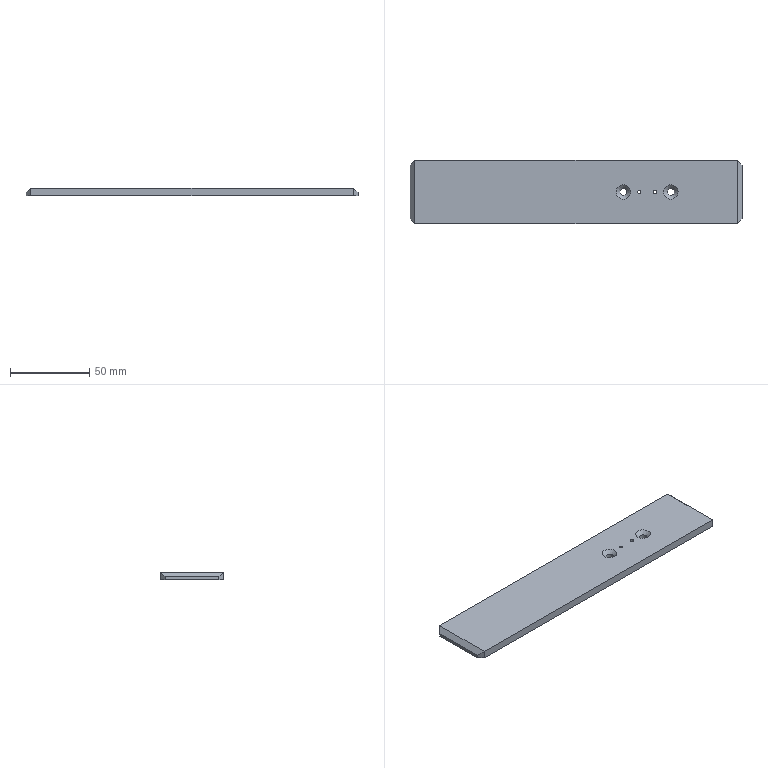Part | STEP file | Tube feed_id782_x_t | 1 solid | 18 faces | box 210 x 40 x 5 mm | volume 41286 mm3 | plane 12 | cylinder 4 | cone 2 | commonest cylinder face diameters 2 x2 4.6 x2
STEP:
#1=CARTESIAN_POINT('',(0.,0.,0.));
#2=DIRECTION('',(0.,0.,1.));
#3=DIRECTION('',(1.,0.,0.));
#4=AXIS2_PLACEMENT_3D('',#1,#2,#3);
#5=CARTESIAN_POINT('',(354.3,10.036,-6.));
#6=VERTEX_POINT('',#5);
#7=CARTESIAN_POINT('',(349.7,10.036,-6.));
#8=VERTEX_POINT('',#7);
#9=CARTESIAN_POINT('',(352.,10.036,-6.));
#10=DIRECTION('',(0.,0.,1.));
#11=DIRECTION('',(1.,0.,0.));
#12=AXIS2_PLACEMENT_3D('',#9,#10,#11);
#13=CIRCLE('',#12,2.3);
#14=CARTESIAN_POINT('',(0.,0.,-6.));
#15=DIRECTION('',(0.,0.,1.));
#16=DIRECTION('',(1.,0.,0.));
#17=AXIS2_PLACEMENT_3D('',#14,#15,#16);
#18=PLANE('',#17);
#19=CARTESIAN_POINT('',(352.,10.036));
#20=DIRECTION('',(1.,0.));
#21=AXIS2_PLACEMENT_2D('',#19,#20);
#22=CIRCLE('',#21,2.3);
#23=(GEOMETRIC_REPRESENTATION_CONTEXT(2)PARAMETRIC_REPRESENTATION_CONTEXT()REPRESENTATION_CONTEXT('',''));
#24=DEFINITIONAL_REPRESENTATION('',(#22),#23);
#25=PCURVE('',#18,#24);
#26=CARTESIAN_POINT('',(352.,10.036,-17.3));
#27=DIRECTION('',(0.,0.,-1.));
#28=DIRECTION('',(-1.,0.,0.));
#29=AXIS2_PLACEMENT_3D('',#26,#27,#28);
#30=CYLINDRICAL_SURFACE('',#29,2.3);
#31=CARTESIAN_POINT('',(3.142,-11.3));
#32=DIRECTION('',(-1.,0.));
#33=VECTOR('',#32,1.);
#34=LINE('',#31,#33);
#35=(GEOMETRIC_REPRESENTATION_CONTEXT(2)PARAMETRIC_REPRESENTATION_CONTEXT()REPRESENTATION_CONTEXT('',''));
#36=DEFINITIONAL_REPRESENTATION('',(#34),#35);
#37=PCURVE('',#30,#36);
#38=SURFACE_CURVE('',#13,(#25,#37),.PCURVE_S1.);
#39=EDGE_CURVE('',#6,#8,#38,.T.);
#40=ORIENTED_EDGE('',*,*,#39,.T.);
#41=CARTESIAN_POINT('',(352.,10.036,-6.));
#42=DIRECTION('',(0.,0.,1.));
#43=DIRECTION('',(1.,0.,0.));
#44=AXIS2_PLACEMENT_3D('',#41,#42,#43);
#45=CIRCLE('',#44,2.3);
#46=CARTESIAN_POINT('',(352.,10.036));
#47=DIRECTION('',(1.,0.));
#48=AXIS2_PLACEMENT_2D('',#46,#47);
#49=CIRCLE('',#48,2.3);
#50=(GEOMETRIC_REPRESENTATION_CONTEXT(2)PARAMETRIC_REPRESENTATION_CONTEXT()REPRESENTATION_CONTEXT('',''));
#51=DEFINITIONAL_REPRESENTATION('',(#49),#50);
#52=PCURVE('',#18,#51);
#53=CARTESIAN_POINT('',(9.425,-11.3));
#54=DIRECTION('',(-1.,0.));
#55=VECTOR('',#54,1.);
#56=LINE('',#53,#55);
#57=(GEOMETRIC_REPRESENTATION_CONTEXT(2)PARAMETRIC_REPRESENTATION_CONTEXT()REPRESENTATION_CONTEXT('',''));
#58=DEFINITIONAL_REPRESENTATION('',(#56),#57);
#59=PCURVE('',#30,#58);
#60=SURFACE_CURVE('',#45,(#52,#59),.PCURVE_S1.);
#61=EDGE_CURVE('',#8,#6,#60,.T.);
#62=ORIENTED_EDGE('',*,*,#61,.T.);
#63=EDGE_LOOP('',(#40,#62));
#64=FACE_BOUND('',#63,.T.);
#65=CARTESIAN_POINT('',(343.,10.036,-6.));
#66=VERTEX_POINT('',#65);
#67=CARTESIAN_POINT('',(342.,10.036,-6.));
#68=DIRECTION('',(0.,0.,1.));
#69=DIRECTION('',(1.,0.,0.));
#70=AXIS2_PLACEMENT_3D('',#67,#68,#69);
#71=CIRCLE('',#70,1.);
#72=CARTESIAN_POINT('',(342.,10.036));
#73=DIRECTION('',(1.,0.));
#74=AXIS2_PLACEMENT_2D('',#72,#73);
#75=CIRCLE('',#74,1.);
#76=(GEOMETRIC_REPRESENTATION_CONTEXT(2)PARAMETRIC_REPRESENTATION_CONTEXT()REPRESENTATION_CONTEXT('',''));
#77=DEFINITIONAL_REPRESENTATION('',(#75),#76);
#78=PCURVE('',#18,#77);
#79=CARTESIAN_POINT('',(342.,10.036,-21.));
#80=DIRECTION('',(0.,0.,-1.));
#81=DIRECTION('',(-1.,0.,0.));
#82=AXIS2_PLACEMENT_3D('',#79,#80,#81);
#83=CYLINDRICAL_SURFACE('',#82,1.);
#84=CARTESIAN_POINT('',(9.425,-15.));
#85=DIRECTION('',(-1.,0.));
#86=VECTOR('',#85,1.);
#87=LINE('',#84,#86);
#88=(GEOMETRIC_REPRESENTATION_CONTEXT(2)PARAMETRIC_REPRESENTATION_CONTEXT()REPRESENTATION_CONTEXT('',''));
#89=DEFINITIONAL_REPRESENTATION('',(#87),#88);
#90=PCURVE('',#83,#89);
#91=SURFACE_CURVE('',#71,(#78,#90),.PCURVE_S1.);
#92=EDGE_CURVE('',#66,#66,#91,.T.);
#93=ORIENTED_EDGE('',*,*,#92,.T.);
#94=EDGE_LOOP('',(#93));
#95=FACE_BOUND('',#94,.T.);
#96=CARTESIAN_POINT('',(333.,10.036,-6.));
#97=VERTEX_POINT('',#96);
#98=CARTESIAN_POINT('',(332.,10.036,-6.));
#99=DIRECTION('',(0.,0.,1.));
#100=DIRECTION('',(1.,0.,0.));
#101=AXIS2_PLACEMENT_3D('',#98,#99,#100);
#102=CIRCLE('',#101,1.);
#103=CARTESIAN_POINT('',(332.,10.036));
#104=DIRECTION('',(1.,0.));
#105=AXIS2_PLACEMENT_2D('',#103,#104);
#106=CIRCLE('',#105,1.);
#107=(GEOMETRIC_REPRESENTATION_CONTEXT(2)PARAMETRIC_REPRESENTATION_CONTEXT()REPRESENTATION_CONTEXT('',''));
#108=DEFINITIONAL_REPRESENTATION('',(#106),#107);
#109=PCURVE('',#18,#108);
#110=CARTESIAN_POINT('',(332.,10.036,-21.));
#111=DIRECTION('',(0.,0.,-1.));
#112=DIRECTION('',(-1.,0.,0.));
#113=AXIS2_PLACEMENT_3D('',#110,#111,#112);
#114=CYLINDRICAL_SURFACE('',#113,1.);
#115=CARTESIAN_POINT('',(9.425,-15.));
#116=DIRECTION('',(-1.,0.));
#117=VECTOR('',#116,1.);
#118=LINE('',#115,#117);
#119=(GEOMETRIC_REPRESENTATION_CONTEXT(2)PARAMETRIC_REPRESENTATION_CONTEXT()REPRESENTATION_CONTEXT('',''));
#120=DEFINITIONAL_REPRESENTATION('',(#118),#119);
#121=PCURVE('',#114,#120);
#122=SURFACE_CURVE('',#102,(#109,#121),.PCURVE_S1.);
#123=EDGE_CURVE('',#97,#97,#122,.T.);
#124=ORIENTED_EDGE('',*,*,#123,.T.);
#125=EDGE_LOOP('',(#124));
#126=FACE_BOUND('',#125,.T.);
#127=CARTESIAN_POINT('',(190.,-9.964,-6.));
#128=VERTEX_POINT('',#127);
#129=CARTESIAN_POINT('',(394.,-9.964,-6.));
#130=VERTEX_POINT('',#129);
#131=CARTESIAN_POINT('',(187.,-9.964,-6.));
#132=DIRECTION('',(1.,0.,0.));
#133=VECTOR('',#132,1.);
#134=LINE('',#131,#133);
#135=CARTESIAN_POINT('',(187.,-9.964));
#136=DIRECTION('',(1.,0.));
#137=VECTOR('',#136,1.);
#138=LINE('',#135,#137);
#139=(GEOMETRIC_REPRESENTATION_CONTEXT(2)PARAMETRIC_REPRESENTATION_CONTEXT()REPRESENTATION_CONTEXT('',''));
#140=DEFINITIONAL_REPRESENTATION('',(#138),#139);
#141=PCURVE('',#18,#140);
#142=CARTESIAN_POINT('',(187.,-9.964,-1.));
#143=DIRECTION('',(0.,1.,0.));
#144=DIRECTION('',(0.,0.,1.));
#145=AXIS2_PLACEMENT_3D('',#142,#143,#144);
#146=PLANE('',#145);
#147=CARTESIAN_POINT('',(-5.,0.));
#148=DIRECTION('',(0.,1.));
#149=VECTOR('',#148,1.);
#150=LINE('',#147,#149);
#151=(GEOMETRIC_REPRESENTATION_CONTEXT(2)PARAMETRIC_REPRESENTATION_CONTEXT()REPRESENTATION_CONTEXT('',''));
#152=DEFINITIONAL_REPRESENTATION('',(#150),#151);
#153=PCURVE('',#146,#152);
#154=SURFACE_CURVE('',#134,(#141,#153),.PCURVE_S1.);
#155=EDGE_CURVE('',#128,#130,#154,.T.);
#156=ORIENTED_EDGE('',*,*,#155,.F.);
#157=CARTESIAN_POINT('',(187.,-6.964,-6.));
#158=VERTEX_POINT('',#157);
#159=CARTESIAN_POINT('',(190.,-9.964,-6.));
#160=DIRECTION('',(-0.7071,0.7071,0.));
#161=VECTOR('',#160,1.);
#162=LINE('',#159,#161);
#163=CARTESIAN_POINT('',(190.,-9.964));
#164=DIRECTION('',(-0.7071,0.7071));
#165=VECTOR('',#164,1.);
#166=LINE('',#163,#165);
#167=(GEOMETRIC_REPRESENTATION_CONTEXT(2)PARAMETRIC_REPRESENTATION_CONTEXT()REPRESENTATION_CONTEXT('',''));
#168=DEFINITIONAL_REPRESENTATION('',(#166),#167);
#169=PCURVE('',#18,#168);
#170=CARTESIAN_POINT('',(190.,-9.964,-1.));
#171=DIRECTION('',(0.7071,0.7071,0.));
#172=DIRECTION('',(0.,0.,-1.));
#173=AXIS2_PLACEMENT_3D('',#170,#171,#172);
#174=PLANE('',#173);
#175=CARTESIAN_POINT('',(5.,0.));
#176=DIRECTION('',(0.,1.));
#177=VECTOR('',#176,1.);
#178=LINE('',#175,#177);
#179=(GEOMETRIC_REPRESENTATION_CONTEXT(2)PARAMETRIC_REPRESENTATION_CONTEXT()REPRESENTATION_CONTEXT('',''));
#180=DEFINITIONAL_REPRESENTATION('',(#178),#179);
#181=PCURVE('',#174,#180);
#182=SURFACE_CURVE('',#162,(#169,#181),.PCURVE_S1.);
#183=EDGE_CURVE('',#128,#158,#182,.T.);
#184=ORIENTED_EDGE('',*,*,#183,.T.);
#185=CARTESIAN_POINT('',(187.,27.036,-6.));
#186=VERTEX_POINT('',#185);
#187=CARTESIAN_POINT('',(187.,30.036,-6.));
#188=DIRECTION('',(0.,-1.,0.));
#189=VECTOR('',#188,1.);
#190=LINE('',#187,#189);
#191=CARTESIAN_POINT('',(187.,30.036));
#192=DIRECTION('',(0.,-1.));
#193=VECTOR('',#192,1.);
#194=LINE('',#191,#193);
#195=(GEOMETRIC_REPRESENTATION_CONTEXT(2)PARAMETRIC_REPRESENTATION_CONTEXT()REPRESENTATION_CONTEXT('',''));
#196=DEFINITIONAL_REPRESENTATION('',(#194),#195);
#197=PCURVE('',#18,#196);
#198=CARTESIAN_POINT('',(187.,30.036,-1.));
#199=DIRECTION('',(1.,0.,0.));
#200=DIRECTION('',(0.,0.,-1.));
#201=AXIS2_PLACEMENT_3D('',#198,#199,#200);
#202=PLANE('',#201);
#203=CARTESIAN_POINT('',(5.,0.));
#204=DIRECTION('',(0.,-1.));
#205=VECTOR('',#204,1.);
#206=LINE('',#203,#205);
#207=(GEOMETRIC_REPRESENTATION_CONTEXT(2)PARAMETRIC_REPRESENTATION_CONTEXT()REPRESENTATION_CONTEXT('',''));
#208=DEFINITIONAL_REPRESENTATION('',(#206),#207);
#209=PCURVE('',#202,#208);
#210=SURFACE_CURVE('',#190,(#197,#209),.PCURVE_S1.);
#211=EDGE_CURVE('',#186,#158,#210,.T.);
#212=ORIENTED_EDGE('',*,*,#211,.F.);
#213=CARTESIAN_POINT('',(190.,30.036,-6.));
#214=VERTEX_POINT('',#213);
#215=CARTESIAN_POINT('',(187.,27.036,-6.));
#216=DIRECTION('',(0.7071,0.7071,0.));
#217=VECTOR('',#216,1.);
#218=LINE('',#215,#217);
#219=CARTESIAN_POINT('',(187.,27.036));
#220=DIRECTION('',(0.7071,0.7071));
#221=VECTOR('',#220,1.);
#222=LINE('',#219,#221);
#223=(GEOMETRIC_REPRESENTATION_CONTEXT(2)PARAMETRIC_REPRESENTATION_CONTEXT()REPRESENTATION_CONTEXT('',''));
#224=DEFINITIONAL_REPRESENTATION('',(#222),#223);
#225=PCURVE('',#18,#224);
#226=CARTESIAN_POINT('',(187.,27.036,-1.));
#227=DIRECTION('',(0.7071,-0.7071,0.));
#228=DIRECTION('',(0.,0.,-1.));
#229=AXIS2_PLACEMENT_3D('',#226,#227,#228);
#230=PLANE('',#229);
#231=CARTESIAN_POINT('',(5.,0.));
#232=DIRECTION('',(0.,1.));
#233=VECTOR('',#232,1.);
#234=LINE('',#231,#233);
#235=(GEOMETRIC_REPRESENTATION_CONTEXT(2)PARAMETRIC_REPRESENTATION_CONTEXT()REPRESENTATION_CONTEXT('',''));
#236=DEFINITIONAL_REPRESENTATION('',(#234),#235);
#237=PCURVE('',#230,#236);
#238=SURFACE_CURVE('',#218,(#225,#237),.PCURVE_S1.);
#239=EDGE_CURVE('',#186,#214,#238,.T.);
#240=ORIENTED_EDGE('',*,*,#239,.T.);
#241=CARTESIAN_POINT('',(394.,30.036,-6.));
#242=VERTEX_POINT('',#241);
#243=CARTESIAN_POINT('',(397.,30.036,-6.));
#244=DIRECTION('',(-1.,0.,0.));
#245=VECTOR('',#244,1.);
#246=LINE('',#243,#245);
#247=CARTESIAN_POINT('',(397.,30.036));
#248=DIRECTION('',(-1.,0.));
#249=VECTOR('',#248,1.);
#250=LINE('',#247,#249);
#251=(GEOMETRIC_REPRESENTATION_CONTEXT(2)PARAMETRIC_REPRESENTATION_CONTEXT()REPRESENTATION_CONTEXT('',''));
#252=DEFINITIONAL_REPRESENTATION('',(#250),#251);
#253=PCURVE('',#18,#252);
#254=CARTESIAN_POINT('',(397.,30.036,-1.));
#255=DIRECTION('',(0.,-1.,0.));
#256=DIRECTION('',(0.,0.,-1.));
#257=AXIS2_PLACEMENT_3D('',#254,#255,#256);
#258=PLANE('',#257);
#259=CARTESIAN_POINT('',(5.,0.));
#260=DIRECTION('',(0.,-1.));
#261=VECTOR('',#260,1.);
#262=LINE('',#259,#261);
#263=(GEOMETRIC_REPRESENTATION_CONTEXT(2)PARAMETRIC_REPRESENTATION_CONTEXT()REPRESENTATION_CONTEXT('',''));
#264=DEFINITIONAL_REPRESENTATION('',(#262),#263);
#265=PCURVE('',#258,#264);
#266=SURFACE_CURVE('',#246,(#253,#265),.PCURVE_S1.);
#267=EDGE_CURVE('',#242,#214,#266,.T.);
#268=ORIENTED_EDGE('',*,*,#267,.F.);
#269=CARTESIAN_POINT('',(397.,27.036,-6.));
#270=VERTEX_POINT('',#269);
#271=CARTESIAN_POINT('',(394.,30.036,-6.));
#272=DIRECTION('',(0.7071,-0.7071,0.));
#273=VECTOR('',#272,1.);
#274=LINE('',#271,#273);
#275=CARTESIAN_POINT('',(394.,30.036));
#276=DIRECTION('',(0.7071,-0.7071));
#277=VECTOR('',#276,1.);
#278=LINE('',#275,#277);
#279=(GEOMETRIC_REPRESENTATION_CONTEXT(2)PARAMETRIC_REPRESENTATION_CONTEXT()REPRESENTATION_CONTEXT('',''));
#280=DEFINITIONAL_REPRESENTATION('',(#278),#279);
#281=PCURVE('',#18,#280);
#282=CARTESIAN_POINT('',(394.,30.036,-1.));
#283=DIRECTION('',(-0.7071,-0.7071,0.));
#284=DIRECTION('',(0.,0.,-1.));
#285=AXIS2_PLACEMENT_3D('',#282,#283,#284);
#286=PLANE('',#285);
#287=CARTESIAN_POINT('',(5.,0.));
#288=DIRECTION('',(0.,1.));
#289=VECTOR('',#288,1.);
#290=LINE('',#287,#289);
#291=(GEOMETRIC_REPRESENTATION_CONTEXT(2)PARAMETRIC_REPRESENTATION_CONTEXT()REPRESENTATION_CONTEXT('',''));
#292=DEFINITIONAL_REPRESENTATION('',(#290),#291);
#293=PCURVE('',#286,#292);
#294=SURFACE_CURVE('',#274,(#281,#293),.PCURVE_S1.);
#295=EDGE_CURVE('',#242,#270,#294,.T.);
#296=ORIENTED_EDGE('',*,*,#295,.T.);
#297=CARTESIAN_POINT('',(397.,-6.964,-6.));
#298=VERTEX_POINT('',#297);
#299=CARTESIAN_POINT('',(397.,-9.964,-6.));
#300=DIRECTION('',(0.,1.,0.));
#301=VECTOR('',#300,1.);
#302=LINE('',#299,#301);
#303=CARTESIAN_POINT('',(397.,-9.964));
#304=DIRECTION('',(0.,1.));
#305=VECTOR('',#304,1.);
#306=LINE('',#303,#305);
#307=(GEOMETRIC_REPRESENTATION_CONTEXT(2)PARAMETRIC_REPRESENTATION_CONTEXT()REPRESENTATION_CONTEXT('',''));
#308=DEFINITIONAL_REPRESENTATION('',(#306),#307);
#309=PCURVE('',#18,#308);
#310=CARTESIAN_POINT('',(397.,-9.964,-1.));
#311=DIRECTION('',(-1.,0.,0.));
#312=DIRECTION('',(0.,0.,1.));
#313=AXIS2_PLACEMENT_3D('',#310,#311,#312);
#314=PLANE('',#313);
#315=CARTESIAN_POINT('',(-5.,0.));
#316=DIRECTION('',(0.,1.));
#317=VECTOR('',#316,1.);
#318=LINE('',#315,#317);
#319=(GEOMETRIC_REPRESENTATION_CONTEXT(2)PARAMETRIC_REPRESENTATION_CONTEXT()REPRESENTATION_CONTEXT('',''));
#320=DEFINITIONAL_REPRESENTATION('',(#318),#319);
#321=PCURVE('',#314,#320);
#322=SURFACE_CURVE('',#302,(#309,#321),.PCURVE_S1.);
#323=EDGE_CURVE('',#298,#270,#322,.T.);
#324=ORIENTED_EDGE('',*,*,#323,.F.);
#325=CARTESIAN_POINT('',(397.,-6.964,-6.));
#326=DIRECTION('',(-0.7071,-0.7071,0.));
#327=VECTOR('',#326,1.);
#328=LINE('',#325,#327);
#329=CARTESIAN_POINT('',(397.,-6.964));
#330=DIRECTION('',(-0.7071,-0.7071));
#331=VECTOR('',#330,1.);
#332=LINE('',#329,#331);
#333=(GEOMETRIC_REPRESENTATION_CONTEXT(2)PARAMETRIC_REPRESENTATION_CONTEXT()REPRESENTATION_CONTEXT('',''));
#334=DEFINITIONAL_REPRESENTATION('',(#332),#333);
#335=PCURVE('',#18,#334);
#336=CARTESIAN_POINT('',(397.,-6.964,-1.));
#337=DIRECTION('',(-0.7071,0.7071,0.));
#338=DIRECTION('',(0.,0.,-1.));
#339=AXIS2_PLACEMENT_3D('',#336,#337,#338);
#340=PLANE('',#339);
#341=CARTESIAN_POINT('',(5.,0.));
#342=DIRECTION('',(0.,1.));
#343=VECTOR('',#342,1.);
#344=LINE('',#341,#343);
#345=(GEOMETRIC_REPRESENTATION_CONTEXT(2)PARAMETRIC_REPRESENTATION_CONTEXT()REPRESENTATION_CONTEXT('',''));
#346=DEFINITIONAL_REPRESENTATION('',(#344),#345);
#347=PCURVE('',#340,#346);
#348=SURFACE_CURVE('',#328,(#335,#347),.PCURVE_S1.);
#349=EDGE_CURVE('',#298,#130,#348,.T.);
#350=ORIENTED_EDGE('',*,*,#349,.T.);
#351=EDGE_LOOP('',(#156,#184,#212,#240,#268,#296,#324,#350));
#352=FACE_BOUND('',#351,.T.);
#353=CARTESIAN_POINT('',(324.3,10.036,-6.));
#354=VERTEX_POINT('',#353);
#355=CARTESIAN_POINT('',(319.7,10.036,-6.));
#356=VERTEX_POINT('',#355);
#357=CARTESIAN_POINT('',(322.,10.036,-6.));
#358=DIRECTION('',(0.,0.,1.));
#359=DIRECTION('',(1.,0.,0.));
#360=AXIS2_PLACEMENT_3D('',#357,#358,#359);
#361=CIRCLE('',#360,2.3);
#362=CARTESIAN_POINT('',(322.,10.036));
#363=DIRECTION('',(1.,0.));
#364=AXIS2_PLACEMENT_2D('',#362,#363);
#365=CIRCLE('',#364,2.3);
#366=(GEOMETRIC_REPRESENTATION_CONTEXT(2)PARAMETRIC_REPRESENTATION_CONTEXT()REPRESENTATION_CONTEXT('',''));
#367=DEFINITIONAL_REPRESENTATION('',(#365),#366);
#368=PCURVE('',#18,#367);
#369=CARTESIAN_POINT('',(322.,10.036,-17.3));
#370=DIRECTION('',(0.,0.,-1.));
#371=DIRECTION('',(-1.,0.,0.));
#372=AXIS2_PLACEMENT_3D('',#369,#370,#371);
#373=CYLINDRICAL_SURFACE('',#372,2.3);
#374=CARTESIAN_POINT('',(3.142,-11.3));
#375=DIRECTION('',(-1.,0.));
#376=VECTOR('',#375,1.);
#377=LINE('',#374,#376);
#378=(GEOMETRIC_REPRESENTATION_CONTEXT(2)PARAMETRIC_REPRESENTATION_CONTEXT()REPRESENTATION_CONTEXT('',''));
#379=DEFINITIONAL_REPRESENTATION('',(#377),#378);
#380=PCURVE('',#373,#379);
#381=SURFACE_CURVE('',#361,(#368,#380),.PCURVE_S1.);
#382=EDGE_CURVE('',#354,#356,#381,.T.);
#383=ORIENTED_EDGE('',*,*,#382,.T.);
#384=CARTESIAN_POINT('',(322.,10.036,-6.));
#385=DIRECTION('',(0.,0.,1.));
#386=DIRECTION('',(1.,0.,0.));
#387=AXIS2_PLACEMENT_3D('',#384,#385,#386);
#388=CIRCLE('',#387,2.3);
#389=CARTESIAN_POINT('',(322.,10.036));
#390=DIRECTION('',(1.,0.));
#391=AXIS2_PLACEMENT_2D('',#389,#390);
#392=CIRCLE('',#391,2.3);
#393=(GEOMETRIC_REPRESENTATION_CONTEXT(2)PARAMETRIC_REPRESENTATION_CONTEXT()REPRESENTATION_CONTEXT('',''));
#394=DEFINITIONAL_REPRESENTATION('',(#392),#393);
#395=PCURVE('',#18,#394);
#396=CARTESIAN_POINT('',(9.425,-11.3));
#397=DIRECTION('',(-1.,0.));
#398=VECTOR('',#397,1.);
#399=LINE('',#396,#398);
#400=(GEOMETRIC_REPRESENTATION_CONTEXT(2)PARAMETRIC_REPRESENTATION_CONTEXT()REPRESENTATION_CONTEXT('',''));
#401=DEFINITIONAL_REPRESENTATION('',(#399),#400);
#402=PCURVE('',#373,#401);
#403=SURFACE_CURVE('',#388,(#395,#402),.PCURVE_S1.);
#404=EDGE_CURVE('',#356,#354,#403,.T.);
#405=ORIENTED_EDGE('',*,*,#404,.T.);
#406=EDGE_LOOP('',(#383,#405));
#407=FACE_BOUND('',#406,.T.);
#408=ADVANCED_FACE('',(#64,#95,#126,#352,#407),#18,.F.);
#409=ORIENTED_EDGE('',*,*,#211,.T.);
#410=CARTESIAN_POINT('',(187.,-6.964,-4.));
#411=VERTEX_POINT('',#410);
#412=CARTESIAN_POINT('',(187.,-6.964,-1.));
#413=DIRECTION('',(0.,0.,1.));
#414=VECTOR('',#413,1.);
#415=LINE('',#412,#414);
#416=CARTESIAN_POINT('',(0.,-37.));
#417=DIRECTION('',(-1.,0.));
#418=VECTOR('',#417,1.);
#419=LINE('',#416,#418);
#420=(GEOMETRIC_REPRESENTATION_CONTEXT(2)PARAMETRIC_REPRESENTATION_CONTEXT()REPRESENTATION_CONTEXT('',''));
#421=DEFINITIONAL_REPRESENTATION('',(#419),#420);
#422=PCURVE('',#202,#421);
#423=CARTESIAN_POINT('',(0.,4.243));
#424=DIRECTION('',(-1.,0.));
#425=VECTOR('',#424,1.);
#426=LINE('',#423,#425);
#427=(GEOMETRIC_REPRESENTATION_CONTEXT(2)PARAMETRIC_REPRESENTATION_CONTEXT()REPRESENTATION_CONTEXT('',''));
#428=DEFINITIONAL_REPRESENTATION('',(#426),#427);
#429=PCURVE('',#174,#428);
#430=SURFACE_CURVE('',#415,(#422,#429),.PCURVE_S1.);
#431=EDGE_CURVE('',#158,#411,#430,.T.);
#432=ORIENTED_EDGE('',*,*,#431,.T.);
#433=CARTESIAN_POINT('',(187.,27.036,-4.));
#434=VERTEX_POINT('',#433);
#435=CARTESIAN_POINT('',(187.,30.036,-4.));
#436=DIRECTION('',(0.,1.,0.));
#437=VECTOR('',#436,1.);
#438=LINE('',#435,#437);
#439=CARTESIAN_POINT('',(3.,0.));
#440=DIRECTION('',(0.,1.));
#441=VECTOR('',#440,1.);
#442=LINE('',#439,#441);
#443=(GEOMETRIC_REPRESENTATION_CONTEXT(2)PARAMETRIC_REPRESENTATION_CONTEXT()REPRESENTATION_CONTEXT('',''));
#444=DEFINITIONAL_REPRESENTATION('',(#442),#443);
#445=PCURVE('',#202,#444);
#446=CARTESIAN_POINT('',(190.,0.,-1.));
#447=DIRECTION('',(-0.7071,0.,0.7071));
#448=DIRECTION('',(0.,1.,0.));
#449=AXIS2_PLACEMENT_3D('',#446,#447,#448);
#450=PLANE('',#449);
#451=CARTESIAN_POINT('',(30.036,4.243));
#452=DIRECTION('',(1.,0.));
#453=VECTOR('',#452,1.);
#454=LINE('',#451,#453);
#455=(GEOMETRIC_REPRESENTATION_CONTEXT(2)PARAMETRIC_REPRESENTATION_CONTEXT()REPRESENTATION_CONTEXT('',''));
#456=DEFINITIONAL_REPRESENTATION('',(#454),#455);
#457=PCURVE('',#450,#456);
#458=SURFACE_CURVE('',#438,(#445,#457),.PCURVE_S1.);
#459=EDGE_CURVE('',#411,#434,#458,.T.);
#460=ORIENTED_EDGE('',*,*,#459,.T.);
#461=CARTESIAN_POINT('',(187.,27.036,-1.));
#462=DIRECTION('',(0.,0.,-1.));
#463=VECTOR('',#462,1.);
#464=LINE('',#461,#463);
#465=CARTESIAN_POINT('',(0.,-3.));
#466=DIRECTION('',(1.,0.));
#467=VECTOR('',#466,1.);
#468=LINE('',#465,#467);
#469=(GEOMETRIC_REPRESENTATION_CONTEXT(2)PARAMETRIC_REPRESENTATION_CONTEXT()REPRESENTATION_CONTEXT('',''));
#470=DEFINITIONAL_REPRESENTATION('',(#468),#469);
#471=PCURVE('',#202,#470);
#472=CARTESIAN_POINT('',(0.,0.));
#473=DIRECTION('',(1.,0.));
#474=VECTOR('',#473,1.);
#475=LINE('',#472,#474);
#476=(GEOMETRIC_REPRESENTATION_CONTEXT(2)PARAMETRIC_REPRESENTATION_CONTEXT()REPRESENTATION_CONTEXT('',''));
#477=DEFINITIONAL_REPRESENTATION('',(#475),#476);
#478=PCURVE('',#230,#477);
#479=SURFACE_CURVE('',#464,(#471,#478),.PCURVE_S1.);
#480=EDGE_CURVE('',#434,#186,#479,.T.);
#481=ORIENTED_EDGE('',*,*,#480,.T.);
#482=EDGE_LOOP('',(#409,#432,#460,#481));
#483=FACE_BOUND('',#482,.T.);
#484=ADVANCED_FACE('',(#483),#202,.F.);
#485=CARTESIAN_POINT('',(190.,-9.964,-1.));
#486=VERTEX_POINT('',#485);
#487=CARTESIAN_POINT('',(394.,-9.964,-1.));
#488=VERTEX_POINT('',#487);
#489=CARTESIAN_POINT('',(187.,-9.964,-1.));
#490=DIRECTION('',(1.,0.,0.));
#491=VECTOR('',#490,1.);
#492=LINE('',#489,#491);
#493=CARTESIAN_POINT('',(0.,0.));
#494=DIRECTION('',(0.,1.));
#495=VECTOR('',#494,1.);
#496=LINE('',#493,#495);
#497=(GEOMETRIC_REPRESENTATION_CONTEXT(2)PARAMETRIC_REPRESENTATION_CONTEXT()REPRESENTATION_CONTEXT('',''));
#498=DEFINITIONAL_REPRESENTATION('',(#496),#497);
#499=PCURVE('',#146,#498);
#500=CARTESIAN_POINT('',(0.,0.,-1.));
#501=DIRECTION('',(0.,0.,1.));
#502=DIRECTION('',(1.,0.,0.));
#503=AXIS2_PLACEMENT_3D('',#500,#501,#502);
#504=PLANE('',#503);
#505=CARTESIAN_POINT('',(187.,-9.964));
#506=DIRECTION('',(1.,0.));
#507=VECTOR('',#506,1.);
#508=LINE('',#505,#507);
#509=(GEOMETRIC_REPRESENTATION_CONTEXT(2)PARAMETRIC_REPRESENTATION_CONTEXT()REPRESENTATION_CONTEXT('',''));
#510=DEFINITIONAL_REPRESENTATION('',(#508),#509);
#511=PCURVE('',#504,#510);
#512=SURFACE_CURVE('',#492,(#499,#511),.PCURVE_S1.);
#513=EDGE_CURVE('',#486,#488,#512,.T.);
#514=ORIENTED_EDGE('',*,*,#513,.F.);
#515=CARTESIAN_POINT('',(190.,-9.964,-1.));
#516=DIRECTION('',(0.,0.,-1.));
#517=VECTOR('',#516,1.);
#518=LINE('',#515,#517);
#519=CARTESIAN_POINT('',(0.,3.));
#520=DIRECTION('',(-1.,0.));
#521=VECTOR('',#520,1.);
#522=LINE('',#519,#521);
#523=(GEOMETRIC_REPRESENTATION_CONTEXT(2)PARAMETRIC_REPRESENTATION_CONTEXT()REPRESENTATION_CONTEXT('',''));
#524=DEFINITIONAL_REPRESENTATION('',(#522),#523);
#525=PCURVE('',#146,#524);
#526=CARTESIAN_POINT('',(0.,0.));
#527=DIRECTION('',(1.,0.));
#528=VECTOR('',#527,1.);
#529=LINE('',#526,#528);
#530=(GEOMETRIC_REPRESENTATION_CONTEXT(2)PARAMETRIC_REPRESENTATION_CONTEXT()REPRESENTATION_CONTEXT('',''));
#531=DEFINITIONAL_REPRESENTATION('',(#529),#530);
#532=PCURVE('',#174,#531);
#533=SURFACE_CURVE('',#518,(#525,#532),.PCURVE_S1.);
#534=EDGE_CURVE('',#486,#128,#533,.T.);
#535=ORIENTED_EDGE('',*,*,#534,.T.);
#536=ORIENTED_EDGE('',*,*,#155,.T.);
#537=CARTESIAN_POINT('',(394.,-9.964,-1.));
#538=DIRECTION('',(0.,0.,1.));
#539=VECTOR('',#538,1.);
#540=LINE('',#537,#539);
#541=CARTESIAN_POINT('',(0.,207.));
#542=DIRECTION('',(1.,0.));
#543=VECTOR('',#542,1.);
#544=LINE('',#541,#543);
#545=(GEOMETRIC_REPRESENTATION_CONTEXT(2)PARAMETRIC_REPRESENTATION_CONTEXT()REPRESENTATION_CONTEXT('',''));
#546=DEFINITIONAL_REPRESENTATION('',(#544),#545);
#547=PCURVE('',#146,#546);
#548=CARTESIAN_POINT('',(0.,4.243));
#549=DIRECTION('',(-1.,0.));
#550=VECTOR('',#549,1.);
#551=LINE('',#548,#550);
#552=(GEOMETRIC_REPRESENTATION_CONTEXT(2)PARAMETRIC_REPRESENTATION_CONTEXT()REPRESENTATION_CONTEXT('',''));
#553=DEFINITIONAL_REPRESENTATION('',(#551),#552);
#554=PCURVE('',#340,#553);
#555=SURFACE_CURVE('',#540,(#547,#554),.PCURVE_S1.);
#556=EDGE_CURVE('',#130,#488,#555,.T.);
#557=ORIENTED_EDGE('',*,*,#556,.T.);
#558=EDGE_LOOP('',(#514,#535,#536,#557));
#559=FACE_BOUND('',#558,.T.);
#560=ADVANCED_FACE('',(#559),#146,.F.);
#561=CARTESIAN_POINT('',(397.,27.036,-4.));
#562=VERTEX_POINT('',#561);
#563=CARTESIAN_POINT('',(397.,-6.964,-4.));
#564=VERTEX_POINT('',#563);
#565=CARTESIAN_POINT('',(397.,-9.964,-4.));
#566=DIRECTION('',(0.,-1.,0.));
#567=VECTOR('',#566,1.);
#568=LINE('',#565,#567);
#569=CARTESIAN_POINT('',(-3.,0.));
#570=DIRECTION('',(0.,-1.));
#571=VECTOR('',#570,1.);
#572=LINE('',#569,#571);
#573=(GEOMETRIC_REPRESENTATION_CONTEXT(2)PARAMETRIC_REPRESENTATION_CONTEXT()REPRESENTATION_CONTEXT('',''));
#574=DEFINITIONAL_REPRESENTATION('',(#572),#573);
#575=PCURVE('',#314,#574);
#576=CARTESIAN_POINT('',(394.,0.,-1.));
#577=DIRECTION('',(0.7071,0.,0.7071));
#578=DIRECTION('',(0.,-1.,0.));
#579=AXIS2_PLACEMENT_3D('',#576,#577,#578);
#580=PLANE('',#579);
#581=CARTESIAN_POINT('',(9.964,4.243));
#582=DIRECTION('',(1.,0.));
#583=VECTOR('',#582,1.);
#584=LINE('',#581,#583);
#585=(GEOMETRIC_REPRESENTATION_CONTEXT(2)PARAMETRIC_REPRESENTATION_CONTEXT()REPRESENTATION_CONTEXT('',''));
#586=DEFINITIONAL_REPRESENTATION('',(#584),#585);
#587=PCURVE('',#580,#586);
#588=SURFACE_CURVE('',#568,(#575,#587),.PCURVE_S1.);
#589=EDGE_CURVE('',#562,#564,#588,.T.);
#590=ORIENTED_EDGE('',*,*,#589,.T.);
#591=CARTESIAN_POINT('',(397.,-6.964,-1.));
#592=DIRECTION('',(0.,0.,-1.));
#593=VECTOR('',#592,1.);
#594=LINE('',#591,#593);
#595=CARTESIAN_POINT('',(0.,3.));
#596=DIRECTION('',(-1.,0.));
#597=VECTOR('',#596,1.);
#598=LINE('',#595,#597);
#599=(GEOMETRIC_REPRESENTATION_CONTEXT(2)PARAMETRIC_REPRESENTATION_CONTEXT()REPRESENTATION_CONTEXT('',''));
#600=DEFINITIONAL_REPRESENTATION('',(#598),#599);
#601=PCURVE('',#314,#600);
#602=CARTESIAN_POINT('',(0.,0.));
#603=DIRECTION('',(1.,0.));
#604=VECTOR('',#603,1.);
#605=LINE('',#602,#604);
#606=(GEOMETRIC_REPRESENTATION_CONTEXT(2)PARAMETRIC_REPRESENTATION_CONTEXT()REPRESENTATION_CONTEXT('',''));
#607=DEFINITIONAL_REPRESENTATION('',(#605),#606);
#608=PCURVE('',#340,#607);
#609=SURFACE_CURVE('',#594,(#601,#608),.PCURVE_S1.);
#610=EDGE_CURVE('',#564,#298,#609,.T.);
#611=ORIENTED_EDGE('',*,*,#610,.T.);
#612=ORIENTED_EDGE('',*,*,#323,.T.);
#613=CARTESIAN_POINT('',(397.,27.036,-1.));
#614=DIRECTION('',(0.,0.,1.));
#615=VECTOR('',#614,1.);
#616=LINE('',#613,#615);
#617=CARTESIAN_POINT('',(0.,37.));
#618=DIRECTION('',(1.,0.));
#619=VECTOR('',#618,1.);
#620=LINE('',#617,#619);
#621=(GEOMETRIC_REPRESENTATION_CONTEXT(2)PARAMETRIC_REPRESENTATION_CONTEXT()REPRESENTATION_CONTEXT('',''));
#622=DEFINITIONAL_REPRESENTATION('',(#620),#621);
#623=PCURVE('',#314,#622);
#624=CARTESIAN_POINT('',(0.,4.243));
#625=DIRECTION('',(-1.,0.));
#626=VECTOR('',#625,1.);
#627=LINE('',#624,#626);
#628=(GEOMETRIC_REPRESENTATION_CONTEXT(2)PARAMETRIC_REPRESENTATION_CONTEXT()REPRESENTATION_CONTEXT('',''));
#629=DEFINITIONAL_REPRESENTATION('',(#627),#628);
#630=PCURVE('',#286,#629);
#631=SURFACE_CURVE('',#616,(#623,#630),.PCURVE_S1.);
#632=EDGE_CURVE('',#270,#562,#631,.T.);
#633=ORIENTED_EDGE('',*,*,#632,.T.);
#634=EDGE_LOOP('',(#590,#611,#612,#633));
#635=FACE_BOUND('',#634,.T.);
#636=ADVANCED_FACE('',(#635),#314,.F.);
#637=ORIENTED_EDGE('',*,*,#267,.T.);
#638=CARTESIAN_POINT('',(190.,30.036,-1.));
#639=VERTEX_POINT('',#638);
#640=CARTESIAN_POINT('',(190.,30.036,-1.));
#641=DIRECTION('',(0.,0.,1.));
#642=VECTOR('',#641,1.);
#643=LINE('',#640,#642);
#644=CARTESIAN_POINT('',(0.,-207.));
#645=DIRECTION('',(-1.,0.));
#646=VECTOR('',#645,1.);
#647=LINE('',#644,#646);
#648=(GEOMETRIC_REPRESENTATION_CONTEXT(2)PARAMETRIC_REPRESENTATION_CONTEXT()REPRESENTATION_CONTEXT('',''));
#649=DEFINITIONAL_REPRESENTATION('',(#647),#648);
#650=PCURVE('',#258,#649);
#651=CARTESIAN_POINT('',(0.,4.243));
#652=DIRECTION('',(-1.,0.));
#653=VECTOR('',#652,1.);
#654=LINE('',#651,#653);
#655=(GEOMETRIC_REPRESENTATION_CONTEXT(2)PARAMETRIC_REPRESENTATION_CONTEXT()REPRESENTATION_CONTEXT('',''));
#656=DEFINITIONAL_REPRESENTATION('',(#654),#655);
#657=PCURVE('',#230,#656);
#658=SURFACE_CURVE('',#643,(#650,#657),.PCURVE_S1.);
#659=EDGE_CURVE('',#214,#639,#658,.T.);
#660=ORIENTED_EDGE('',*,*,#659,.T.);
#661=CARTESIAN_POINT('',(394.,30.036,-1.));
#662=VERTEX_POINT('',#661);
#663=CARTESIAN_POINT('',(397.,30.036,-1.));
#664=DIRECTION('',(-1.,0.,0.));
#665=VECTOR('',#664,1.);
#666=LINE('',#663,#665);
#667=CARTESIAN_POINT('',(0.,0.));
#668=DIRECTION('',(0.,-1.));
#669=VECTOR('',#668,1.);
#670=LINE('',#667,#669);
#671=(GEOMETRIC_REPRESENTATION_CONTEXT(2)PARAMETRIC_REPRESENTATION_CONTEXT()REPRESENTATION_CONTEXT('',''));
#672=DEFINITIONAL_REPRESENTATION('',(#670),#671);
#673=PCURVE('',#258,#672);
#674=CARTESIAN_POINT('',(397.,30.036));
#675=DIRECTION('',(-1.,0.));
#676=VECTOR('',#675,1.);
#677=LINE('',#674,#676);
#678=(GEOMETRIC_REPRESENTATION_CONTEXT(2)PARAMETRIC_REPRESENTATION_CONTEXT()REPRESENTATION_CONTEXT('',''));
#679=DEFINITIONAL_REPRESENTATION('',(#677),#678);
#680=PCURVE('',#504,#679);
#681=SURFACE_CURVE('',#666,(#673,#680),.PCURVE_S1.);
#682=EDGE_CURVE('',#662,#639,#681,.T.);
#683=ORIENTED_EDGE('',*,*,#682,.F.);
#684=CARTESIAN_POINT('',(394.,30.036,-1.));
#685=DIRECTION('',(0.,0.,-1.));
#686=VECTOR('',#685,1.);
#687=LINE('',#684,#686);
#688=CARTESIAN_POINT('',(0.,-3.));
#689=DIRECTION('',(1.,0.));
#690=VECTOR('',#689,1.);
#691=LINE('',#688,#690);
#692=(GEOMETRIC_REPRESENTATION_CONTEXT(2)PARAMETRIC_REPRESENTATION_CONTEXT()REPRESENTATION_CONTEXT('',''));
#693=DEFINITIONAL_REPRESENTATION('',(#691),#692);
#694=PCURVE('',#258,#693);
#695=CARTESIAN_POINT('',(0.,0.));
#696=DIRECTION('',(1.,0.));
#697=VECTOR('',#696,1.);
#698=LINE('',#695,#697);
#699=(GEOMETRIC_REPRESENTATION_CONTEXT(2)PARAMETRIC_REPRESENTATION_CONTEXT()REPRESENTATION_CONTEXT('',''));
#700=DEFINITIONAL_REPRESENTATION('',(#698),#699);
#701=PCURVE('',#286,#700);
#702=SURFACE_CURVE('',#687,(#694,#701),.PCURVE_S1.);
#703=EDGE_CURVE('',#662,#242,#702,.T.);
#704=ORIENTED_EDGE('',*,*,#703,.T.);
#705=EDGE_LOOP('',(#637,#660,#683,#704));
#706=FACE_BOUND('',#705,.T.);
#707=ADVANCED_FACE('',(#706),#258,.F.);
#708=CARTESIAN_POINT('',(347.4,10.036,-1.));
#709=VERTEX_POINT('',#708);
#710=CARTESIAN_POINT('',(352.,10.036,-1.));
#711=DIRECTION('',(0.,0.,-1.));
#712=DIRECTION('',(-1.,0.,0.));
#713=AXIS2_PLACEMENT_3D('',#710,#711,#712);
#714=CIRCLE('',#713,4.6);
#715=CARTESIAN_POINT('',(347.4,10.036));
#716=CARTESIAN_POINT('',(347.4,18.003));
#717=CARTESIAN_POINT('',(354.3,14.019));
#718=CARTESIAN_POINT('',(361.2,10.036));
#719=CARTESIAN_POINT('',(354.3,6.052));
#720=CARTESIAN_POINT('',(347.4,2.068));
#721=CARTESIAN_POINT('',(347.4,10.036));
#722=(BOUNDED_CURVE()B_SPLINE_CURVE(2,(#715,#716,#717,#718,#719,#720,#721),.UNSPECIFIED.,.T.,.F.)B_SPLINE_CURVE_WITH_KNOTS((1,2,2,2,2,1),(-2.094,0.,2.094,4.189,6.283,8.378),.UNSPECIFIED.)CURVE()GEOMETRIC_REPRESENTATION_ITEM()RATIONAL_B_SPLINE_CURVE((1.,0.5,1.,0.5,1.,0.5,1.))REPRESENTATION_ITEM(''));
#723=(GEOMETRIC_REPRESENTATION_CONTEXT(2)PARAMETRIC_REPRESENTATION_CONTEXT()REPRESENTATION_CONTEXT('',''));
#724=DEFINITIONAL_REPRESENTATION('',(#722),#723);
#725=PCURVE('',#504,#724);
#726=CARTESIAN_POINT('',(352.,10.036,-3.3));
#727=DIRECTION('',(0.,0.,1.));
#728=DIRECTION('',(1.,0.,0.));
#729=AXIS2_PLACEMENT_3D('',#726,#727,#728);
#730=CONICAL_SURFACE('',#729,2.3,0.7854);
#731=CARTESIAN_POINT('',(9.425,2.3));
#732=DIRECTION('',(-1.,0.));
#733=VECTOR('',#732,1.);
#734=LINE('',#731,#733);
#735=(GEOMETRIC_REPRESENTATION_CONTEXT(2)PARAMETRIC_REPRESENTATION_CONTEXT()REPRESENTATION_CONTEXT('',''));
#736=DEFINITIONAL_REPRESENTATION('',(#734),#735);
#737=PCURVE('',#730,#736);
#738=SURFACE_CURVE('',#714,(#725,#737),.PCURVE_S1.);
#739=EDGE_CURVE('',#709,#709,#738,.T.);
#740=ORIENTED_EDGE('',*,*,#739,.T.);
#741=EDGE_LOOP('',(#740));
#742=FACE_BOUND('',#741,.T.);
#743=CARTESIAN_POINT('',(317.4,10.036,-1.));
#744=VERTEX_POINT('',#743);
#745=CARTESIAN_POINT('',(322.,10.036,-1.));
#746=DIRECTION('',(0.,0.,-1.));
#747=DIRECTION('',(-1.,0.,0.));
#748=AXIS2_PLACEMENT_3D('',#745,#746,#747);
#749=CIRCLE('',#748,4.6);
#750=CARTESIAN_POINT('',(317.4,10.036));
#751=CARTESIAN_POINT('',(317.4,18.003));
#752=CARTESIAN_POINT('',(324.3,14.019));
#753=CARTESIAN_POINT('',(331.2,10.036));
#754=CARTESIAN_POINT('',(324.3,6.052));
#755=CARTESIAN_POINT('',(317.4,2.068));
#756=CARTESIAN_POINT('',(317.4,10.036));
#757=(BOUNDED_CURVE()B_SPLINE_CURVE(2,(#750,#751,#752,#753,#754,#755,#756),.UNSPECIFIED.,.T.,.F.)B_SPLINE_CURVE_WITH_KNOTS((1,2,2,2,2,1),(-2.094,0.,2.094,4.189,6.283,8.378),.UNSPECIFIED.)CURVE()GEOMETRIC_REPRESENTATION_ITEM()RATIONAL_B_SPLINE_CURVE((1.,0.5,1.,0.5,1.,0.5,1.))REPRESENTATION_ITEM(''));
#758=(GEOMETRIC_REPRESENTATION_CONTEXT(2)PARAMETRIC_REPRESENTATION_CONTEXT()REPRESENTATION_CONTEXT('',''));
#759=DEFINITIONAL_REPRESENTATION('',(#757),#758);
#760=PCURVE('',#504,#759);
#761=CARTESIAN_POINT('',(322.,10.036,-3.3));
#762=DIRECTION('',(0.,0.,1.));
#763=DIRECTION('',(1.,0.,0.));
#764=AXIS2_PLACEMENT_3D('',#761,#762,#763);
#765=CONICAL_SURFACE('',#764,2.3,0.7854);
#766=CARTESIAN_POINT('',(9.425,2.3));
#767=DIRECTION('',(-1.,0.));
#768=VECTOR('',#767,1.);
#769=LINE('',#766,#768);
#770=(GEOMETRIC_REPRESENTATION_CONTEXT(2)PARAMETRIC_REPRESENTATION_CONTEXT()REPRESENTATION_CONTEXT('',''));
#771=DEFINITIONAL_REPRESENTATION('',(#769),#770);
#772=PCURVE('',#765,#771);
#773=SURFACE_CURVE('',#749,(#760,#772),.PCURVE_S1.);
#774=EDGE_CURVE('',#744,#744,#773,.T.);
#775=ORIENTED_EDGE('',*,*,#774,.T.);
#776=EDGE_LOOP('',(#775));
#777=FACE_BOUND('',#776,.T.);
#778=CARTESIAN_POINT('',(343.,10.036,-1.));
#779=VERTEX_POINT('',#778);
#780=CARTESIAN_POINT('',(342.,10.036,-1.));
#781=DIRECTION('',(0.,0.,1.));
#782=DIRECTION('',(1.,0.,0.));
#783=AXIS2_PLACEMENT_3D('',#780,#781,#782);
#784=CIRCLE('',#783,1.);
#785=CARTESIAN_POINT('',(342.,10.036));
#786=DIRECTION('',(1.,0.));
#787=AXIS2_PLACEMENT_2D('',#785,#786);
#788=CIRCLE('',#787,1.);
#789=(GEOMETRIC_REPRESENTATION_CONTEXT(2)PARAMETRIC_REPRESENTATION_CONTEXT()REPRESENTATION_CONTEXT('',''));
#790=DEFINITIONAL_REPRESENTATION('',(#788),#789);
#791=PCURVE('',#504,#790);
#792=CARTESIAN_POINT('',(9.425,-20.));
#793=DIRECTION('',(-1.,0.));
#794=VECTOR('',#793,1.);
#795=LINE('',#792,#794);
#796=(GEOMETRIC_REPRESENTATION_CONTEXT(2)PARAMETRIC_REPRESENTATION_CONTEXT()REPRESENTATION_CONTEXT('',''));
#797=DEFINITIONAL_REPRESENTATION('',(#795),#796);
#798=PCURVE('',#83,#797);
#799=SURFACE_CURVE('',#784,(#791,#798),.PCURVE_S1.);
#800=EDGE_CURVE('',#779,#779,#799,.T.);
#801=ORIENTED_EDGE('',*,*,#800,.F.);
#802=EDGE_LOOP('',(#801));
#803=FACE_BOUND('',#802,.T.);
#804=CARTESIAN_POINT('',(333.,10.036,-1.));
#805=VERTEX_POINT('',#804);
#806=CARTESIAN_POINT('',(332.,10.036,-1.));
#807=DIRECTION('',(0.,0.,1.));
#808=DIRECTION('',(1.,0.,0.));
#809=AXIS2_PLACEMENT_3D('',#806,#807,#808);
#810=CIRCLE('',#809,1.);
#811=CARTESIAN_POINT('',(332.,10.036));
#812=DIRECTION('',(1.,0.));
#813=AXIS2_PLACEMENT_2D('',#811,#812);
#814=CIRCLE('',#813,1.);
#815=(GEOMETRIC_REPRESENTATION_CONTEXT(2)PARAMETRIC_REPRESENTATION_CONTEXT()REPRESENTATION_CONTEXT('',''));
#816=DEFINITIONAL_REPRESENTATION('',(#814),#815);
#817=PCURVE('',#504,#816);
#818=CARTESIAN_POINT('',(9.425,-20.));
#819=DIRECTION('',(-1.,0.));
#820=VECTOR('',#819,1.);
#821=LINE('',#818,#820);
#822=(GEOMETRIC_REPRESENTATION_CONTEXT(2)PARAMETRIC_REPRESENTATION_CONTEXT()REPRESENTATION_CONTEXT('',''));
#823=DEFINITIONAL_REPRESENTATION('',(#821),#822);
#824=PCURVE('',#114,#823);
#825=SURFACE_CURVE('',#810,(#817,#824),.PCURVE_S1.);
#826=EDGE_CURVE('',#805,#805,#825,.T.);
#827=ORIENTED_EDGE('',*,*,#826,.F.);
#828=EDGE_LOOP('',(#827));
#829=FACE_BOUND('',#828,.T.);
#830=ORIENTED_EDGE('',*,*,#682,.T.);
#831=CARTESIAN_POINT('',(190.,-9.964,-1.));
#832=DIRECTION('',(0.,-1.,0.));
#833=VECTOR('',#832,1.);
#834=LINE('',#831,#833);
#835=CARTESIAN_POINT('',(190.,-9.964));
#836=DIRECTION('',(0.,-1.));
#837=VECTOR('',#836,1.);
#838=LINE('',#835,#837);
#839=(GEOMETRIC_REPRESENTATION_CONTEXT(2)PARAMETRIC_REPRESENTATION_CONTEXT()REPRESENTATION_CONTEXT('',''));
#840=DEFINITIONAL_REPRESENTATION('',(#838),#839);
#841=PCURVE('',#504,#840);
#842=CARTESIAN_POINT('',(-9.964,0.));
#843=DIRECTION('',(-1.,0.));
#844=VECTOR('',#843,1.);
#845=LINE('',#842,#844);
#846=(GEOMETRIC_REPRESENTATION_CONTEXT(2)PARAMETRIC_REPRESENTATION_CONTEXT()REPRESENTATION_CONTEXT('',''));
#847=DEFINITIONAL_REPRESENTATION('',(#845),#846);
#848=PCURVE('',#450,#847);
#849=SURFACE_CURVE('',#834,(#841,#848),.PCURVE_S1.);
#850=EDGE_CURVE('',#639,#486,#849,.T.);
#851=ORIENTED_EDGE('',*,*,#850,.T.);
#852=ORIENTED_EDGE('',*,*,#513,.T.);
#853=CARTESIAN_POINT('',(394.,30.036,-1.));
#854=DIRECTION('',(0.,1.,0.));
#855=VECTOR('',#854,1.);
#856=LINE('',#853,#855);
#857=CARTESIAN_POINT('',(394.,30.036));
#858=DIRECTION('',(0.,1.));
#859=VECTOR('',#858,1.);
#860=LINE('',#857,#859);
#861=(GEOMETRIC_REPRESENTATION_CONTEXT(2)PARAMETRIC_REPRESENTATION_CONTEXT()REPRESENTATION_CONTEXT('',''));
#862=DEFINITIONAL_REPRESENTATION('',(#860),#861);
#863=PCURVE('',#504,#862);
#864=CARTESIAN_POINT('',(-30.036,0.));
#865=DIRECTION('',(-1.,0.));
#866=VECTOR('',#865,1.);
#867=LINE('',#864,#866);
#868=(GEOMETRIC_REPRESENTATION_CONTEXT(2)PARAMETRIC_REPRESENTATION_CONTEXT()REPRESENTATION_CONTEXT('',''));
#869=DEFINITIONAL_REPRESENTATION('',(#867),#868);
#870=PCURVE('',#580,#869);
#871=SURFACE_CURVE('',#856,(#863,#870),.PCURVE_S1.);
#872=EDGE_CURVE('',#488,#662,#871,.T.);
#873=ORIENTED_EDGE('',*,*,#872,.T.);
#874=EDGE_LOOP('',(#830,#851,#852,#873));
#875=FACE_BOUND('',#874,.T.);
#876=ADVANCED_FACE('',(#742,#777,#803,#829,#875),#504,.T.);
#877=ORIENTED_EDGE('',*,*,#239,.F.);
#878=ORIENTED_EDGE('',*,*,#480,.F.);
#879=CARTESIAN_POINT('',(188.,28.036,-3.));
#880=DIRECTION('',(-0.5774,-0.5774,-0.5774));
#881=VECTOR('',#880,1.);
#882=LINE('',#879,#881);
#883=CARTESIAN_POINT('',(2.,1.414));
#884=DIRECTION('',(0.5774,-0.8165));
#885=VECTOR('',#884,1.);
#886=LINE('',#883,#885);
#887=(GEOMETRIC_REPRESENTATION_CONTEXT(2)PARAMETRIC_REPRESENTATION_CONTEXT()REPRESENTATION_CONTEXT('',''));
#888=DEFINITIONAL_REPRESENTATION('',(#886),#887);
#889=PCURVE('',#230,#888);
#890=CARTESIAN_POINT('',(28.036,2.828));
#891=DIRECTION('',(-0.5774,0.8165));
#892=VECTOR('',#891,1.);
#893=LINE('',#890,#892);
#894=(GEOMETRIC_REPRESENTATION_CONTEXT(2)PARAMETRIC_REPRESENTATION_CONTEXT()REPRESENTATION_CONTEXT('',''));
#895=DEFINITIONAL_REPRESENTATION('',(#893),#894);
#896=PCURVE('',#450,#895);
#897=SURFACE_CURVE('',#882,(#889,#896),.PCURVE_S1.);
#898=EDGE_CURVE('',#639,#434,#897,.T.);
#899=ORIENTED_EDGE('',*,*,#898,.F.);
#900=ORIENTED_EDGE('',*,*,#659,.F.);
#901=EDGE_LOOP('',(#877,#878,#899,#900));
#902=FACE_BOUND('',#901,.T.);
#903=ADVANCED_FACE('',(#902),#230,.F.);
#904=ORIENTED_EDGE('',*,*,#898,.T.);
#905=ORIENTED_EDGE('',*,*,#459,.F.);
#906=CARTESIAN_POINT('',(186.679,-6.643,-4.321));
#907=DIRECTION('',(-0.5774,0.5774,-0.5774));
#908=VECTOR('',#907,1.);
#909=LINE('',#906,#908);
#910=CARTESIAN_POINT('',(-6.643,4.697));
#911=DIRECTION('',(0.5774,0.8165));
#912=VECTOR('',#911,1.);
#913=LINE('',#910,#912);
#914=(GEOMETRIC_REPRESENTATION_CONTEXT(2)PARAMETRIC_REPRESENTATION_CONTEXT()REPRESENTATION_CONTEXT('',''));
#915=DEFINITIONAL_REPRESENTATION('',(#913),#914);
#916=PCURVE('',#450,#915);
#917=CARTESIAN_POINT('',(3.321,4.697));
#918=DIRECTION('',(0.5774,0.8165));
#919=VECTOR('',#918,1.);
#920=LINE('',#917,#919);
#921=(GEOMETRIC_REPRESENTATION_CONTEXT(2)PARAMETRIC_REPRESENTATION_CONTEXT()REPRESENTATION_CONTEXT('',''));
#922=DEFINITIONAL_REPRESENTATION('',(#920),#921);
#923=PCURVE('',#174,#922);
#924=SURFACE_CURVE('',#909,(#916,#923),.PCURVE_S1.);
#925=EDGE_CURVE('',#486,#411,#924,.T.);
#926=ORIENTED_EDGE('',*,*,#925,.F.);
#927=ORIENTED_EDGE('',*,*,#850,.F.);
#928=EDGE_LOOP('',(#904,#905,#926,#927));
#929=FACE_BOUND('',#928,.T.);
#930=ADVANCED_FACE('',(#929),#450,.T.);
#931=ORIENTED_EDGE('',*,*,#925,.T.);
#932=ORIENTED_EDGE('',*,*,#431,.F.);
#933=ORIENTED_EDGE('',*,*,#183,.F.);
#934=ORIENTED_EDGE('',*,*,#534,.F.);
#935=EDGE_LOOP('',(#931,#932,#933,#934));
#936=FACE_BOUND('',#935,.T.);
#937=ADVANCED_FACE('',(#936),#174,.F.);
#938=ORIENTED_EDGE('',*,*,#295,.F.);
#939=ORIENTED_EDGE('',*,*,#703,.F.);
#940=CARTESIAN_POINT('',(404.012,20.024,-11.012));
#941=DIRECTION('',(-0.5774,0.5774,0.5774));
#942=VECTOR('',#941,1.);
#943=LINE('',#940,#942);
#944=CARTESIAN_POINT('',(10.012,14.159));
#945=DIRECTION('',(-0.5774,-0.8165));
#946=VECTOR('',#945,1.);
#947=LINE('',#944,#946);
#948=(GEOMETRIC_REPRESENTATION_CONTEXT(2)PARAMETRIC_REPRESENTATION_CONTEXT()REPRESENTATION_CONTEXT('',''));
#949=DEFINITIONAL_REPRESENTATION('',(#947),#948);
#950=PCURVE('',#286,#949);
#951=CARTESIAN_POINT('',(-20.024,14.159));
#952=DIRECTION('',(-0.5774,-0.8165));
#953=VECTOR('',#952,1.);
#954=LINE('',#951,#953);
#955=(GEOMETRIC_REPRESENTATION_CONTEXT(2)PARAMETRIC_REPRESENTATION_CONTEXT()REPRESENTATION_CONTEXT('',''));
#956=DEFINITIONAL_REPRESENTATION('',(#954),#955);
#957=PCURVE('',#580,#956);
#958=SURFACE_CURVE('',#943,(#950,#957),.PCURVE_S1.);
#959=EDGE_CURVE('',#562,#662,#958,.T.);
#960=ORIENTED_EDGE('',*,*,#959,.F.);
#961=ORIENTED_EDGE('',*,*,#632,.F.);
#962=EDGE_LOOP('',(#938,#939,#960,#961));
#963=FACE_BOUND('',#962,.T.);
#964=ADVANCED_FACE('',(#963),#286,.F.);
#965=ORIENTED_EDGE('',*,*,#959,.T.);
#966=ORIENTED_EDGE('',*,*,#872,.F.);
#967=CARTESIAN_POINT('',(397.321,-6.643,-4.321));
#968=DIRECTION('',(-0.5774,-0.5774,0.5774));
#969=VECTOR('',#968,1.);
#970=LINE('',#967,#969);
#971=CARTESIAN_POINT('',(6.643,4.697));
#972=DIRECTION('',(0.5774,-0.8165));
#973=VECTOR('',#972,1.);
#974=LINE('',#971,#973);
#975=(GEOMETRIC_REPRESENTATION_CONTEXT(2)PARAMETRIC_REPRESENTATION_CONTEXT()REPRESENTATION_CONTEXT('',''));
#976=DEFINITIONAL_REPRESENTATION('',(#974),#975);
#977=PCURVE('',#580,#976);
#978=CARTESIAN_POINT('',(3.321,-0.4546));
#979=DIRECTION('',(-0.5774,0.8165));
#980=VECTOR('',#979,1.);
#981=LINE('',#978,#980);
#982=(GEOMETRIC_REPRESENTATION_CONTEXT(2)PARAMETRIC_REPRESENTATION_CONTEXT()REPRESENTATION_CONTEXT('',''));
#983=DEFINITIONAL_REPRESENTATION('',(#981),#982);
#984=PCURVE('',#340,#983);
#985=SURFACE_CURVE('',#970,(#977,#984),.PCURVE_S1.);
#986=EDGE_CURVE('',#564,#488,#985,.T.);
#987=ORIENTED_EDGE('',*,*,#986,.F.);
#988=ORIENTED_EDGE('',*,*,#589,.F.);
#989=EDGE_LOOP('',(#965,#966,#987,#988));
#990=FACE_BOUND('',#989,.T.);
#991=ADVANCED_FACE('',(#990),#580,.T.);
#992=ORIENTED_EDGE('',*,*,#986,.T.);
#993=ORIENTED_EDGE('',*,*,#556,.F.);
#994=ORIENTED_EDGE('',*,*,#349,.F.);
#995=ORIENTED_EDGE('',*,*,#610,.F.);
#996=EDGE_LOOP('',(#992,#993,#994,#995));
#997=FACE_BOUND('',#996,.T.);
#998=ADVANCED_FACE('',(#997),#340,.F.);
#999=ORIENTED_EDGE('',*,*,#123,.T.);
#1000=CARTESIAN_POINT('',(333.,10.036,-1.));
#1001=CARTESIAN_POINT('',(333.,10.036,-6.));
#1002=B_SPLINE_CURVE_WITH_KNOTS('',1,(#1000,#1001),.UNSPECIFIED.,.F.,.F.,(2,2),(-20.,-15.),.PIECEWISE_BEZIER_KNOTS.);
#1003=CARTESIAN_POINT('',(3.142,0.));
#1004=DIRECTION('',(0.,1.));
#1005=VECTOR('',#1004,1.);
#1006=LINE('',#1003,#1005);
#1007=(GEOMETRIC_REPRESENTATION_CONTEXT(2)PARAMETRIC_REPRESENTATION_CONTEXT()REPRESENTATION_CONTEXT('',''));
#1008=DEFINITIONAL_REPRESENTATION('',(#1006),#1007);
#1009=PCURVE('',#114,#1008);
#1010=CARTESIAN_POINT('',(9.425,0.));
#1011=DIRECTION('',(0.,1.));
#1012=VECTOR('',#1011,1.);
#1013=LINE('',#1010,#1012);
#1014=(GEOMETRIC_REPRESENTATION_CONTEXT(2)PARAMETRIC_REPRESENTATION_CONTEXT()REPRESENTATION_CONTEXT('',''));
#1015=DEFINITIONAL_REPRESENTATION('',(#1013),#1014);
#1016=PCURVE('',#114,#1015);
#1017=SEAM_CURVE('',#1002,(#1009,#1016),.PCURVE_S1.);
#1018=EDGE_CURVE('',#805,#97,#1017,.T.);
#1019=ORIENTED_EDGE('',*,*,#1018,.F.);
#1020=ORIENTED_EDGE('',*,*,#826,.F.);
#1021=ORIENTED_EDGE('',*,*,#1018,.T.);
#1022=EDGE_LOOP('',(#999,#1019,#1020,#1021));
#1023=FACE_BOUND('',#1022,.F.);
#1024=ADVANCED_FACE('',(#1023),#114,.F.);
#1025=ORIENTED_EDGE('',*,*,#92,.T.);
#1026=CARTESIAN_POINT('',(343.,10.036,-1.));
#1027=CARTESIAN_POINT('',(343.,10.036,-6.));
#1028=B_SPLINE_CURVE_WITH_KNOTS('',1,(#1026,#1027),.UNSPECIFIED.,.F.,.F.,(2,2),(-20.,-15.),.PIECEWISE_BEZIER_KNOTS.);
#1029=CARTESIAN_POINT('',(3.142,0.));
#1030=DIRECTION('',(0.,1.));
#1031=VECTOR('',#1030,1.);
#1032=LINE('',#1029,#1031);
#1033=(GEOMETRIC_REPRESENTATION_CONTEXT(2)PARAMETRIC_REPRESENTATION_CONTEXT()REPRESENTATION_CONTEXT('',''));
#1034=DEFINITIONAL_REPRESENTATION('',(#1032),#1033);
#1035=PCURVE('',#83,#1034);
#1036=CARTESIAN_POINT('',(9.425,0.));
#1037=DIRECTION('',(0.,1.));
#1038=VECTOR('',#1037,1.);
#1039=LINE('',#1036,#1038);
#1040=(GEOMETRIC_REPRESENTATION_CONTEXT(2)PARAMETRIC_REPRESENTATION_CONTEXT()REPRESENTATION_CONTEXT('',''));
#1041=DEFINITIONAL_REPRESENTATION('',(#1039),#1040);
#1042=PCURVE('',#83,#1041);
#1043=SEAM_CURVE('',#1028,(#1035,#1042),.PCURVE_S1.);
#1044=EDGE_CURVE('',#779,#66,#1043,.T.);
#1045=ORIENTED_EDGE('',*,*,#1044,.F.);
#1046=ORIENTED_EDGE('',*,*,#800,.F.);
#1047=ORIENTED_EDGE('',*,*,#1044,.T.);
#1048=EDGE_LOOP('',(#1025,#1045,#1046,#1047));
#1049=FACE_BOUND('',#1048,.F.);
#1050=ADVANCED_FACE('',(#1049),#83,.F.);
#1051=ORIENTED_EDGE('',*,*,#774,.T.);
#1052=CARTESIAN_POINT('',(319.7,10.036,-3.3));
#1053=VERTEX_POINT('',#1052);
#1054=CARTESIAN_POINT('',(319.7,10.036,-3.3));
#1055=CARTESIAN_POINT('',(317.4,10.036,-1.));
#1056=B_SPLINE_CURVE_WITH_KNOTS('',1,(#1054,#1055),.UNSPECIFIED.,.F.,.F.,(2,2),(0.,3.253),.PIECEWISE_BEZIER_KNOTS.);
#1057=CARTESIAN_POINT('',(3.142,0.));
#1058=DIRECTION('',(0.,1.));
#1059=VECTOR('',#1058,1.);
#1060=LINE('',#1057,#1059);
#1061=(GEOMETRIC_REPRESENTATION_CONTEXT(2)PARAMETRIC_REPRESENTATION_CONTEXT()REPRESENTATION_CONTEXT('',''));
#1062=DEFINITIONAL_REPRESENTATION('',(#1060),#1061);
#1063=PCURVE('',#765,#1062);
#1064=CARTESIAN_POINT('',(9.425,0.));
#1065=DIRECTION('',(0.,1.));
#1066=VECTOR('',#1065,1.);
#1067=LINE('',#1064,#1066);
#1068=(GEOMETRIC_REPRESENTATION_CONTEXT(2)PARAMETRIC_REPRESENTATION_CONTEXT()REPRESENTATION_CONTEXT('',''));
#1069=DEFINITIONAL_REPRESENTATION('',(#1067),#1068);
#1070=PCURVE('',#765,#1069);
#1071=SEAM_CURVE('',#1056,(#1063,#1070),.PCURVE_S1.);
#1072=EDGE_CURVE('',#1053,#744,#1071,.T.);
#1073=ORIENTED_EDGE('',*,*,#1072,.F.);
#1074=CARTESIAN_POINT('',(322.,10.036,-3.3));
#1075=DIRECTION('',(0.,0.,1.));
#1076=DIRECTION('',(-1.,0.,0.));
#1077=AXIS2_PLACEMENT_3D('',#1074,#1075,#1076);
#1078=CIRCLE('',#1077,2.3);
#1079=CARTESIAN_POINT('',(3.142,0.));
#1080=DIRECTION('',(1.,0.));
#1081=VECTOR('',#1080,1.);
#1082=LINE('',#1079,#1081);
#1083=(GEOMETRIC_REPRESENTATION_CONTEXT(2)PARAMETRIC_REPRESENTATION_CONTEXT()REPRESENTATION_CONTEXT('',''));
#1084=DEFINITIONAL_REPRESENTATION('',(#1082),#1083);
#1085=PCURVE('',#765,#1084);
#1086=CARTESIAN_POINT('',(6.283,-14.));
#1087=DIRECTION('',(-1.,0.));
#1088=VECTOR('',#1087,1.);
#1089=LINE('',#1086,#1088);
#1090=(GEOMETRIC_REPRESENTATION_CONTEXT(2)PARAMETRIC_REPRESENTATION_CONTEXT()REPRESENTATION_CONTEXT('',''));
#1091=DEFINITIONAL_REPRESENTATION('',(#1089),#1090);
#1092=PCURVE('',#373,#1091);
#1093=SURFACE_CURVE('',#1078,(#1085,#1092),.PCURVE_S1.);
#1094=EDGE_CURVE('',#1053,#1053,#1093,.T.);
#1095=ORIENTED_EDGE('',*,*,#1094,.T.);
#1096=ORIENTED_EDGE('',*,*,#1072,.T.);
#1097=EDGE_LOOP('',(#1051,#1073,#1095,#1096));
#1098=FACE_BOUND('',#1097,.F.);
#1099=ADVANCED_FACE('',(#1098),#765,.F.);
#1100=ORIENTED_EDGE('',*,*,#1094,.F.);
#1101=CARTESIAN_POINT('',(319.7,10.036,-3.3));
#1102=CARTESIAN_POINT('',(319.7,10.036,-6.));
#1103=B_SPLINE_CURVE_WITH_KNOTS('',1,(#1101,#1102),.UNSPECIFIED.,.F.,.F.,(2,2),(-14.,-11.3),.PIECEWISE_BEZIER_KNOTS.);
#1104=CARTESIAN_POINT('',(6.283,0.));
#1105=DIRECTION('',(0.,1.));
#1106=VECTOR('',#1105,1.);
#1107=LINE('',#1104,#1106);
#1108=(GEOMETRIC_REPRESENTATION_CONTEXT(2)PARAMETRIC_REPRESENTATION_CONTEXT()REPRESENTATION_CONTEXT('',''));
#1109=DEFINITIONAL_REPRESENTATION('',(#1107),#1108);
#1110=PCURVE('',#373,#1109);
#1111=CARTESIAN_POINT('',(0.,0.));
#1112=DIRECTION('',(0.,1.));
#1113=VECTOR('',#1112,1.);
#1114=LINE('',#1111,#1113);
#1115=(GEOMETRIC_REPRESENTATION_CONTEXT(2)PARAMETRIC_REPRESENTATION_CONTEXT()REPRESENTATION_CONTEXT('',''));
#1116=DEFINITIONAL_REPRESENTATION('',(#1114),#1115);
#1117=PCURVE('',#373,#1116);
#1118=SEAM_CURVE('',#1103,(#1110,#1117),.PCURVE_S1.);
#1119=EDGE_CURVE('',#1053,#356,#1118,.T.);
#1120=ORIENTED_EDGE('',*,*,#1119,.T.);
#1121=ORIENTED_EDGE('',*,*,#404,.T.);
#1122=ORIENTED_EDGE('',*,*,#382,.T.);
#1123=ORIENTED_EDGE('',*,*,#1119,.F.);
#1124=EDGE_LOOP('',(#1100,#1120,#1121,#1122,#1123));
#1125=FACE_BOUND('',#1124,.F.);
#1126=ADVANCED_FACE('',(#1125),#373,.F.);
#1127=ORIENTED_EDGE('',*,*,#739,.T.);
#1128=CARTESIAN_POINT('',(349.7,10.036,-3.3));
#1129=VERTEX_POINT('',#1128);
#1130=CARTESIAN_POINT('',(349.7,10.036,-3.3));
#1131=CARTESIAN_POINT('',(347.4,10.036,-1.));
#1132=B_SPLINE_CURVE_WITH_KNOTS('',1,(#1130,#1131),.UNSPECIFIED.,.F.,.F.,(2,2),(0.,3.253),.PIECEWISE_BEZIER_KNOTS.);
#1133=CARTESIAN_POINT('',(3.142,0.));
#1134=DIRECTION('',(0.,1.));
#1135=VECTOR('',#1134,1.);
#1136=LINE('',#1133,#1135);
#1137=(GEOMETRIC_REPRESENTATION_CONTEXT(2)PARAMETRIC_REPRESENTATION_CONTEXT()REPRESENTATION_CONTEXT('',''));
#1138=DEFINITIONAL_REPRESENTATION('',(#1136),#1137);
#1139=PCURVE('',#730,#1138);
#1140=CARTESIAN_POINT('',(9.425,0.));
#1141=DIRECTION('',(0.,1.));
#1142=VECTOR('',#1141,1.);
#1143=LINE('',#1140,#1142);
#1144=(GEOMETRIC_REPRESENTATION_CONTEXT(2)PARAMETRIC_REPRESENTATION_CONTEXT()REPRESENTATION_CONTEXT('',''));
#1145=DEFINITIONAL_REPRESENTATION('',(#1143),#1144);
#1146=PCURVE('',#730,#1145);
#1147=SEAM_CURVE('',#1132,(#1139,#1146),.PCURVE_S1.);
#1148=EDGE_CURVE('',#1129,#709,#1147,.T.);
#1149=ORIENTED_EDGE('',*,*,#1148,.F.);
#1150=CARTESIAN_POINT('',(352.,10.036,-3.3));
#1151=DIRECTION('',(0.,0.,1.));
#1152=DIRECTION('',(-1.,0.,0.));
#1153=AXIS2_PLACEMENT_3D('',#1150,#1151,#1152);
#1154=CIRCLE('',#1153,2.3);
#1155=CARTESIAN_POINT('',(3.142,0.));
#1156=DIRECTION('',(1.,0.));
#1157=VECTOR('',#1156,1.);
#1158=LINE('',#1155,#1157);
#1159=(GEOMETRIC_REPRESENTATION_CONTEXT(2)PARAMETRIC_REPRESENTATION_CONTEXT()REPRESENTATION_CONTEXT('',''));
#1160=DEFINITIONAL_REPRESENTATION('',(#1158),#1159);
#1161=PCURVE('',#730,#1160);
#1162=CARTESIAN_POINT('',(6.283,-14.));
#1163=DIRECTION('',(-1.,0.));
#1164=VECTOR('',#1163,1.);
#1165=LINE('',#1162,#1164);
#1166=(GEOMETRIC_REPRESENTATION_CONTEXT(2)PARAMETRIC_REPRESENTATION_CONTEXT()REPRESENTATION_CONTEXT('',''));
#1167=DEFINITIONAL_REPRESENTATION('',(#1165),#1166);
#1168=PCURVE('',#30,#1167);
#1169=SURFACE_CURVE('',#1154,(#1161,#1168),.PCURVE_S1.);
#1170=EDGE_CURVE('',#1129,#1129,#1169,.T.);
#1171=ORIENTED_EDGE('',*,*,#1170,.T.);
#1172=ORIENTED_EDGE('',*,*,#1148,.T.);
#1173=EDGE_LOOP('',(#1127,#1149,#1171,#1172));
#1174=FACE_BOUND('',#1173,.F.);
#1175=ADVANCED_FACE('',(#1174),#730,.F.);
#1176=ORIENTED_EDGE('',*,*,#1170,.F.);
#1177=CARTESIAN_POINT('',(349.7,10.036,-3.3));
#1178=CARTESIAN_POINT('',(349.7,10.036,-6.));
#1179=B_SPLINE_CURVE_WITH_KNOTS('',1,(#1177,#1178),.UNSPECIFIED.,.F.,.F.,(2,2),(-14.,-11.3),.PIECEWISE_BEZIER_KNOTS.);
#1180=CARTESIAN_POINT('',(6.283,0.));
#1181=DIRECTION('',(0.,1.));
#1182=VECTOR('',#1181,1.);
#1183=LINE('',#1180,#1182);
#1184=(GEOMETRIC_REPRESENTATION_CONTEXT(2)PARAMETRIC_REPRESENTATION_CONTEXT()REPRESENTATION_CONTEXT('',''));
#1185=DEFINITIONAL_REPRESENTATION('',(#1183),#1184);
#1186=PCURVE('',#30,#1185);
#1187=CARTESIAN_POINT('',(0.,0.));
#1188=DIRECTION('',(0.,1.));
#1189=VECTOR('',#1188,1.);
#1190=LINE('',#1187,#1189);
#1191=(GEOMETRIC_REPRESENTATION_CONTEXT(2)PARAMETRIC_REPRESENTATION_CONTEXT()REPRESENTATION_CONTEXT('',''));
#1192=DEFINITIONAL_REPRESENTATION('',(#1190),#1191);
#1193=PCURVE('',#30,#1192);
#1194=SEAM_CURVE('',#1179,(#1186,#1193),.PCURVE_S1.);
#1195=EDGE_CURVE('',#1129,#8,#1194,.T.);
#1196=ORIENTED_EDGE('',*,*,#1195,.T.);
#1197=ORIENTED_EDGE('',*,*,#61,.T.);
#1198=ORIENTED_EDGE('',*,*,#39,.T.);
#1199=ORIENTED_EDGE('',*,*,#1195,.F.);
#1200=EDGE_LOOP('',(#1176,#1196,#1197,#1198,#1199));
#1201=FACE_BOUND('',#1200,.F.);
#1202=ADVANCED_FACE('',(#1201),#30,.F.);
#1203=CLOSED_SHELL('',(#408,#484,#560,#636,#707,#876,#903,#930,#937,#964,#991,#998,#1024,#1050,#1099,#1126,#1175,#1202));
#1204=MANIFOLD_SOLID_BREP('',#1203);
#1205=(LENGTH_UNIT()NAMED_UNIT(*)SI_UNIT(.MILLI.,.METRE.));
#1206=UNCERTAINTY_MEASURE_WITH_UNIT(LENGTH_MEASURE(0.000002),#1205,'','');
#1207=(NAMED_UNIT(*)PLANE_ANGLE_UNIT()SI_UNIT($,.RADIAN.));
#1208=(NAMED_UNIT(*)SI_UNIT($,.STERADIAN.)SOLID_ANGLE_UNIT());
#1209=(GEOMETRIC_REPRESENTATION_CONTEXT(3)GLOBAL_UNCERTAINTY_ASSIGNED_CONTEXT((#1206))GLOBAL_UNIT_ASSIGNED_CONTEXT((#1205,#1207,#1208))REPRESENTATION_CONTEXT('',''));
#1210=ADVANCED_BREP_SHAPE_REPRESENTATION('',(#4,#1204),#1209);